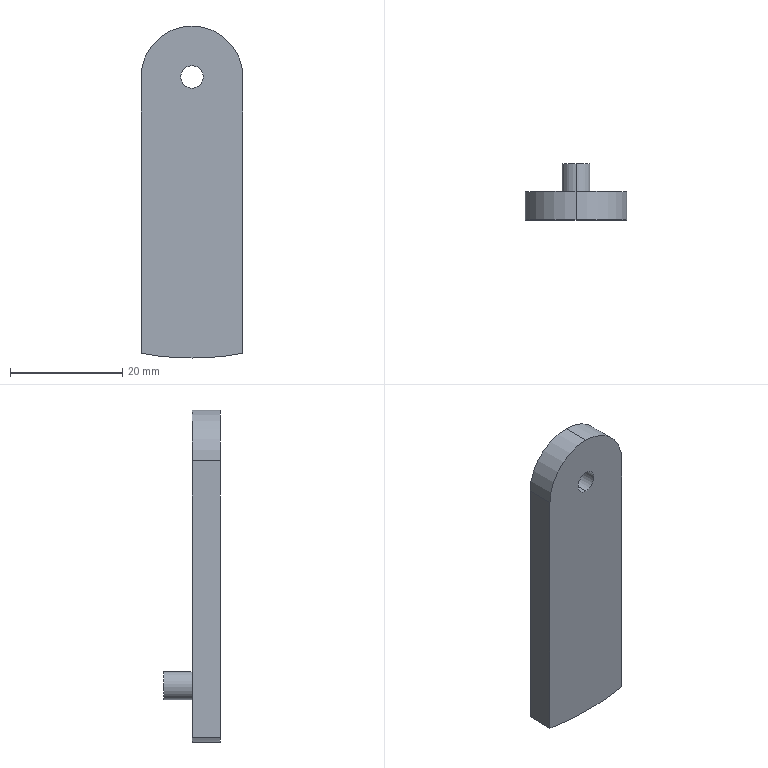Part | SolidWorks | features ICE 3, Extrusion 1 | 1 solid | 13 faces | box 18.129 x 10 x 59.065 mm | volume 5188 mm3 | cylinder 8 | plane 5 | commonest cylinder face diameters 4 x2 5 x2 18.129 x2 100 x2
STEP:
#1=CARTESIAN_POINT('',(0.,5.,-2.));
#2=VERTEX_POINT('',#1);
#3=CARTESIAN_POINT('',(0.,5.,2.));
#4=VERTEX_POINT('',#3);
#5=CARTESIAN_POINT('',(0.,5.,0.));
#6=DIRECTION('',(0.,1.,0.));
#7=DIRECTION('',(0.,0.,1.));
#8=AXIS2_PLACEMENT_3D('',#5,#6,#7);
#9=CIRCLE('',#8,2.);
#10=EDGE_CURVE('',#2,#4,#9,.T.);
#11=ORIENTED_EDGE('',*,*,#10,.T.);
#12=CARTESIAN_POINT('',(0.,0.,2.));
#13=VERTEX_POINT('',#12);
#14=CARTESIAN_POINT('',(0.,10.,2.));
#15=DIRECTION('',(0.,-1.,0.));
#16=VECTOR('',#15,1000.);
#17=LINE('',#14,#16);
#18=EDGE_CURVE('',#4,#13,#17,.T.);
#19=ORIENTED_EDGE('',*,*,#18,.T.);
#20=CARTESIAN_POINT('',(0.,0.,-2.));
#21=VERTEX_POINT('',#20);
#22=CARTESIAN_POINT('',(0.,0.,0.));
#23=DIRECTION('',(0.,-1.,0.));
#24=DIRECTION('',(0.,0.,-1.));
#25=AXIS2_PLACEMENT_3D('',#22,#23,#24);
#26=CIRCLE('',#25,2.);
#27=EDGE_CURVE('',#13,#21,#26,.T.);
#28=ORIENTED_EDGE('',*,*,#27,.T.);
#29=CARTESIAN_POINT('',(0.,10.,-2.));
#30=DIRECTION('',(0.,-1.,0.));
#31=VECTOR('',#30,1000.);
#32=LINE('',#29,#31);
#33=EDGE_CURVE('',#2,#21,#32,.T.);
#34=ORIENTED_EDGE('',*,*,#33,.F.);
#35=EDGE_LOOP('',(#11,#19,#28,#34));
#36=FACE_OUTER_BOUND('',#35,.T.);
#37=CARTESIAN_POINT('',(0.,10.,0.));
#38=DIRECTION('',(0.,-1.,0.));
#39=DIRECTION('',(0.,0.,-1.));
#40=AXIS2_PLACEMENT_3D('',#37,#38,#39);
#41=CYLINDRICAL_SURFACE('',#40,2.);
#42=ADVANCED_FACE('',(#36),#41,.F.);
#43=CARTESIAN_POINT('',(0.,0.,9.065));
#44=VERTEX_POINT('',#43);
#45=CARTESIAN_POINT('',(-9.065,0.,0.));
#46=VERTEX_POINT('',#45);
#47=CARTESIAN_POINT('',(0.,0.,0.));
#48=DIRECTION('',(0.,-1.,0.));
#49=DIRECTION('',(0.,0.,1.));
#50=AXIS2_PLACEMENT_3D('',#47,#48,#49);
#51=CIRCLE('',#50,9.065);
#52=EDGE_CURVE('',#44,#46,#51,.T.);
#53=ORIENTED_EDGE('',*,*,#52,.F.);
#54=CARTESIAN_POINT('',(0.,5.,9.065));
#55=VERTEX_POINT('',#54);
#56=CARTESIAN_POINT('',(0.,-6.,9.065));
#57=DIRECTION('',(0.,1.,0.));
#58=VECTOR('',#57,1000.);
#59=LINE('',#56,#58);
#60=EDGE_CURVE('',#44,#55,#59,.T.);
#61=ORIENTED_EDGE('',*,*,#60,.T.);
#62=CARTESIAN_POINT('',(-9.065,5.,0.));
#63=VERTEX_POINT('',#62);
#64=CARTESIAN_POINT('',(0.,5.,0.));
#65=DIRECTION('',(0.,-1.,0.));
#66=DIRECTION('',(0.,0.,1.));
#67=AXIS2_PLACEMENT_3D('',#64,#65,#66);
#68=CIRCLE('',#67,9.065);
#69=EDGE_CURVE('',#55,#63,#68,.T.);
#70=ORIENTED_EDGE('',*,*,#69,.T.);
#71=CARTESIAN_POINT('',(-9.065,-6.,0.));
#72=DIRECTION('',(0.,1.,0.));
#73=VECTOR('',#72,1000.);
#74=LINE('',#71,#73);
#75=EDGE_CURVE('',#46,#63,#74,.T.);
#76=ORIENTED_EDGE('',*,*,#75,.F.);
#77=EDGE_LOOP('',(#53,#61,#70,#76));
#78=FACE_OUTER_BOUND('',#77,.T.);
#79=CARTESIAN_POINT('',(0.,-6.,0.));
#80=DIRECTION('',(0.,1.,0.));
#81=DIRECTION('',(0.,0.,1.));
#82=AXIS2_PLACEMENT_3D('',#79,#80,#81);
#83=CYLINDRICAL_SURFACE('',#82,9.065);
#84=ADVANCED_FACE('',(#78),#83,.T.);
#85=CARTESIAN_POINT('',(0.,10.,-37.5));
#86=VERTEX_POINT('',#85);
#87=CARTESIAN_POINT('',(0.,10.,-42.5));
#88=VERTEX_POINT('',#87);
#89=CARTESIAN_POINT('',(0.,10.,-40.));
#90=DIRECTION('',(0.,1.,0.));
#91=DIRECTION('',(0.,0.,1.));
#92=AXIS2_PLACEMENT_3D('',#89,#90,#91);
#93=CIRCLE('',#92,2.5);
#94=EDGE_CURVE('',#86,#88,#93,.T.);
#95=ORIENTED_EDGE('',*,*,#94,.F.);
#96=CARTESIAN_POINT('',(0.,5.,-37.5));
#97=VERTEX_POINT('',#96);
#98=CARTESIAN_POINT('',(0.,10.,-37.5));
#99=DIRECTION('',(0.,-1.,0.));
#100=VECTOR('',#99,1000.);
#101=LINE('',#98,#100);
#102=EDGE_CURVE('',#86,#97,#101,.T.);
#103=ORIENTED_EDGE('',*,*,#102,.T.);
#104=CARTESIAN_POINT('',(0.,5.,-42.5));
#105=VERTEX_POINT('',#104);
#106=CARTESIAN_POINT('',(0.,5.,-40.));
#107=DIRECTION('',(0.,-1.,0.));
#108=DIRECTION('',(0.,0.,1.));
#109=AXIS2_PLACEMENT_3D('',#106,#107,#108);
#110=CIRCLE('',#109,2.5);
#111=EDGE_CURVE('',#105,#97,#110,.T.);
#112=ORIENTED_EDGE('',*,*,#111,.F.);
#113=CARTESIAN_POINT('',(0.,10.,-42.5));
#114=DIRECTION('',(0.,-1.,0.));
#115=VECTOR('',#114,1000.);
#116=LINE('',#113,#115);
#117=EDGE_CURVE('',#88,#105,#116,.T.);
#118=ORIENTED_EDGE('',*,*,#117,.F.);
#119=EDGE_LOOP('',(#95,#103,#112,#118));
#120=FACE_OUTER_BOUND('',#119,.T.);
#121=CARTESIAN_POINT('',(0.,10.,-40.));
#122=DIRECTION('',(0.,-1.,0.));
#123=DIRECTION('',(0.,0.,-1.));
#124=AXIS2_PLACEMENT_3D('',#121,#122,#123);
#125=CYLINDRICAL_SURFACE('',#124,2.5);
#126=ADVANCED_FACE('',(#120),#125,.T.);
#127=CARTESIAN_POINT('',(0.,5.,-50.));
#128=VERTEX_POINT('',#127);
#129=CARTESIAN_POINT('',(-9.065,5.,-49.171));
#130=VERTEX_POINT('',#129);
#131=CARTESIAN_POINT('',(0.,5.,0.));
#132=DIRECTION('',(0.,1.,0.));
#133=DIRECTION('',(0.,0.,1.));
#134=AXIS2_PLACEMENT_3D('',#131,#132,#133);
#135=CIRCLE('',#134,50.);
#136=EDGE_CURVE('',#128,#130,#135,.T.);
#137=ORIENTED_EDGE('',*,*,#136,.F.);
#138=CARTESIAN_POINT('',(0.,0.,-50.));
#139=VERTEX_POINT('',#138);
#140=CARTESIAN_POINT('',(0.,5.,-50.));
#141=DIRECTION('',(0.,-1.,0.));
#142=VECTOR('',#141,1000.);
#143=LINE('',#140,#142);
#144=EDGE_CURVE('',#128,#139,#143,.T.);
#145=ORIENTED_EDGE('',*,*,#144,.T.);
#146=CARTESIAN_POINT('',(-9.065,0.,-49.171));
#147=VERTEX_POINT('',#146);
#148=CARTESIAN_POINT('',(0.,0.,0.));
#149=DIRECTION('',(0.,1.,0.));
#150=DIRECTION('',(0.,0.,1.));
#151=AXIS2_PLACEMENT_3D('',#148,#149,#150);
#152=CIRCLE('',#151,50.);
#153=EDGE_CURVE('',#139,#147,#152,.T.);
#154=ORIENTED_EDGE('',*,*,#153,.T.);
#155=CARTESIAN_POINT('',(-9.065,-6.,-49.171));
#156=DIRECTION('',(0.,1.,0.));
#157=VECTOR('',#156,1000.);
#158=LINE('',#155,#157);
#159=EDGE_CURVE('',#147,#130,#158,.T.);
#160=ORIENTED_EDGE('',*,*,#159,.T.);
#161=EDGE_LOOP('',(#137,#145,#154,#160));
#162=FACE_OUTER_BOUND('',#161,.T.);
#163=CARTESIAN_POINT('',(0.,5.,0.));
#164=DIRECTION('',(0.,-1.,0.));
#165=DIRECTION('',(0.,0.,-1.));
#166=AXIS2_PLACEMENT_3D('',#163,#164,#165);
#167=CYLINDRICAL_SURFACE('',#166,50.);
#168=ADVANCED_FACE('',(#162),#167,.T.);
#169=ORIENTED_EDGE('',*,*,#144,.F.);
#170=CARTESIAN_POINT('',(9.065,5.,-49.171));
#171=VERTEX_POINT('',#170);
#172=CARTESIAN_POINT('',(0.,5.,0.));
#173=DIRECTION('',(0.,1.,0.));
#174=DIRECTION('',(0.,0.,1.));
#175=AXIS2_PLACEMENT_3D('',#172,#173,#174);
#176=CIRCLE('',#175,50.);
#177=EDGE_CURVE('',#171,#128,#176,.T.);
#178=ORIENTED_EDGE('',*,*,#177,.F.);
#179=CARTESIAN_POINT('',(9.065,0.,-49.171));
#180=VERTEX_POINT('',#179);
#181=CARTESIAN_POINT('',(9.065,-6.,-49.171));
#182=DIRECTION('',(0.,1.,0.));
#183=VECTOR('',#182,1000.);
#184=LINE('',#181,#183);
#185=EDGE_CURVE('',#180,#171,#184,.T.);
#186=ORIENTED_EDGE('',*,*,#185,.F.);
#187=CARTESIAN_POINT('',(0.,0.,0.));
#188=DIRECTION('',(0.,1.,0.));
#189=DIRECTION('',(0.,0.,1.));
#190=AXIS2_PLACEMENT_3D('',#187,#188,#189);
#191=CIRCLE('',#190,50.);
#192=EDGE_CURVE('',#180,#139,#191,.T.);
#193=ORIENTED_EDGE('',*,*,#192,.T.);
#194=EDGE_LOOP('',(#169,#178,#186,#193));
#195=FACE_OUTER_BOUND('',#194,.T.);
#196=CARTESIAN_POINT('',(0.,5.,0.));
#197=DIRECTION('',(0.,-1.,0.));
#198=DIRECTION('',(0.,0.,-1.));
#199=AXIS2_PLACEMENT_3D('',#196,#197,#198);
#200=CYLINDRICAL_SURFACE('',#199,50.);
#201=ADVANCED_FACE('',(#195),#200,.T.);
#202=ORIENTED_EDGE('',*,*,#10,.F.);
#203=CARTESIAN_POINT('',(0.,5.,0.));
#204=DIRECTION('',(0.,1.,0.));
#205=DIRECTION('',(0.,0.,1.));
#206=AXIS2_PLACEMENT_3D('',#203,#204,#205);
#207=CIRCLE('',#206,2.);
#208=EDGE_CURVE('',#4,#2,#207,.T.);
#209=ORIENTED_EDGE('',*,*,#208,.F.);
#210=EDGE_LOOP('',(#202,#209));
#211=FACE_BOUND('',#210,.T.);
#212=CARTESIAN_POINT('',(-9.065,5.,-20.));
#213=DIRECTION('',(0.,0.,-1.));
#214=VECTOR('',#213,1000.);
#215=LINE('',#212,#214);
#216=EDGE_CURVE('',#63,#130,#215,.T.);
#217=ORIENTED_EDGE('',*,*,#216,.F.);
#218=ORIENTED_EDGE('',*,*,#69,.F.);
#219=CARTESIAN_POINT('',(9.065,5.,0.));
#220=VERTEX_POINT('',#219);
#221=CARTESIAN_POINT('',(0.,5.,0.));
#222=DIRECTION('',(0.,-1.,0.));
#223=DIRECTION('',(0.,0.,1.));
#224=AXIS2_PLACEMENT_3D('',#221,#222,#223);
#225=CIRCLE('',#224,9.065);
#226=EDGE_CURVE('',#220,#55,#225,.T.);
#227=ORIENTED_EDGE('',*,*,#226,.F.);
#228=CARTESIAN_POINT('',(9.065,5.,-20.));
#229=DIRECTION('',(0.,0.,1.));
#230=VECTOR('',#229,1000.);
#231=LINE('',#228,#230);
#232=EDGE_CURVE('',#171,#220,#231,.T.);
#233=ORIENTED_EDGE('',*,*,#232,.F.);
#234=ORIENTED_EDGE('',*,*,#177,.T.);
#235=ORIENTED_EDGE('',*,*,#136,.T.);
#236=EDGE_LOOP('',(#217,#218,#227,#233,#234,#235));
#237=FACE_OUTER_BOUND('',#236,.T.);
#238=ORIENTED_EDGE('',*,*,#111,.T.);
#239=CARTESIAN_POINT('',(0.,5.,-40.));
#240=DIRECTION('',(0.,-1.,0.));
#241=DIRECTION('',(0.,0.,1.));
#242=AXIS2_PLACEMENT_3D('',#239,#240,#241);
#243=CIRCLE('',#242,2.5);
#244=EDGE_CURVE('',#97,#105,#243,.T.);
#245=ORIENTED_EDGE('',*,*,#244,.T.);
#246=EDGE_LOOP('',(#238,#245));
#247=FACE_BOUND('',#246,.T.);
#248=CARTESIAN_POINT('',(0.,5.,0.));
#249=DIRECTION('',(0.,1.,0.));
#250=DIRECTION('',(0.,0.,1.));
#251=AXIS2_PLACEMENT_3D('',#248,#249,#250);
#252=PLANE('',#251);
#253=ADVANCED_FACE('',(#211,#237,#247),#252,.T.);
#254=CARTESIAN_POINT('',(0.,0.,0.));
#255=DIRECTION('',(0.,-1.,0.));
#256=DIRECTION('',(0.,0.,-1.));
#257=AXIS2_PLACEMENT_3D('',#254,#255,#256);
#258=CIRCLE('',#257,2.);
#259=EDGE_CURVE('',#21,#13,#258,.T.);
#260=ORIENTED_EDGE('',*,*,#259,.F.);
#261=ORIENTED_EDGE('',*,*,#27,.F.);
#262=EDGE_LOOP('',(#260,#261));
#263=FACE_BOUND('',#262,.T.);
#264=CARTESIAN_POINT('',(9.065,0.,0.));
#265=VERTEX_POINT('',#264);
#266=CARTESIAN_POINT('',(0.,0.,0.));
#267=DIRECTION('',(0.,-1.,0.));
#268=DIRECTION('',(0.,0.,1.));
#269=AXIS2_PLACEMENT_3D('',#266,#267,#268);
#270=CIRCLE('',#269,9.065);
#271=EDGE_CURVE('',#265,#44,#270,.T.);
#272=ORIENTED_EDGE('',*,*,#271,.T.);
#273=ORIENTED_EDGE('',*,*,#52,.T.);
#274=CARTESIAN_POINT('',(-9.065,0.,0.));
#275=DIRECTION('',(0.,0.,-1.));
#276=VECTOR('',#275,1000.);
#277=LINE('',#274,#276);
#278=EDGE_CURVE('',#46,#147,#277,.T.);
#279=ORIENTED_EDGE('',*,*,#278,.T.);
#280=ORIENTED_EDGE('',*,*,#153,.F.);
#281=ORIENTED_EDGE('',*,*,#192,.F.);
#282=CARTESIAN_POINT('',(9.065,0.,0.));
#283=DIRECTION('',(0.,0.,1.));
#284=VECTOR('',#283,1000.);
#285=LINE('',#282,#284);
#286=EDGE_CURVE('',#180,#265,#285,.T.);
#287=ORIENTED_EDGE('',*,*,#286,.T.);
#288=EDGE_LOOP('',(#272,#273,#279,#280,#281,#287));
#289=FACE_OUTER_BOUND('',#288,.T.);
#290=CARTESIAN_POINT('',(0.,0.,0.));
#291=DIRECTION('',(0.,1.,0.));
#292=DIRECTION('',(0.,0.,1.));
#293=AXIS2_PLACEMENT_3D('',#290,#291,#292);
#294=PLANE('',#293);
#295=ADVANCED_FACE('',(#263,#289),#294,.F.);
#296=ORIENTED_EDGE('',*,*,#102,.F.);
#297=CARTESIAN_POINT('',(0.,10.,-40.));
#298=DIRECTION('',(0.,1.,0.));
#299=DIRECTION('',(0.,0.,1.));
#300=AXIS2_PLACEMENT_3D('',#297,#298,#299);
#301=CIRCLE('',#300,2.5);
#302=EDGE_CURVE('',#88,#86,#301,.T.);
#303=ORIENTED_EDGE('',*,*,#302,.F.);
#304=ORIENTED_EDGE('',*,*,#117,.T.);
#305=ORIENTED_EDGE('',*,*,#244,.F.);
#306=EDGE_LOOP('',(#296,#303,#304,#305));
#307=FACE_OUTER_BOUND('',#306,.T.);
#308=CARTESIAN_POINT('',(0.,10.,-40.));
#309=DIRECTION('',(0.,-1.,0.));
#310=DIRECTION('',(0.,0.,-1.));
#311=AXIS2_PLACEMENT_3D('',#308,#309,#310);
#312=CYLINDRICAL_SURFACE('',#311,2.5);
#313=ADVANCED_FACE('',(#307),#312,.T.);
#314=ORIENTED_EDGE('',*,*,#302,.T.);
#315=ORIENTED_EDGE('',*,*,#94,.T.);
#316=EDGE_LOOP('',(#314,#315));
#317=FACE_OUTER_BOUND('',#316,.T.);
#318=CARTESIAN_POINT('',(0.,10.,0.));
#319=DIRECTION('',(0.,1.,0.));
#320=DIRECTION('',(0.,0.,1.));
#321=AXIS2_PLACEMENT_3D('',#318,#319,#320);
#322=PLANE('',#321);
#323=ADVANCED_FACE('',(#317),#322,.T.);
#324=ORIENTED_EDGE('',*,*,#75,.T.);
#325=ORIENTED_EDGE('',*,*,#216,.T.);
#326=ORIENTED_EDGE('',*,*,#159,.F.);
#327=ORIENTED_EDGE('',*,*,#278,.F.);
#328=EDGE_LOOP('',(#324,#325,#326,#327));
#329=FACE_OUTER_BOUND('',#328,.T.);
#330=CARTESIAN_POINT('',(-9.065,-6.,-20.));
#331=DIRECTION('',(1.,0.,0.));
#332=DIRECTION('',(0.,0.,-1.));
#333=AXIS2_PLACEMENT_3D('',#330,#331,#332);
#334=PLANE('',#333);
#335=ADVANCED_FACE('',(#329),#334,.F.);
#336=ORIENTED_EDGE('',*,*,#60,.F.);
#337=ORIENTED_EDGE('',*,*,#271,.F.);
#338=CARTESIAN_POINT('',(9.065,-6.,0.));
#339=DIRECTION('',(0.,1.,0.));
#340=VECTOR('',#339,1000.);
#341=LINE('',#338,#340);
#342=EDGE_CURVE('',#265,#220,#341,.T.);
#343=ORIENTED_EDGE('',*,*,#342,.T.);
#344=ORIENTED_EDGE('',*,*,#226,.T.);
#345=EDGE_LOOP('',(#336,#337,#343,#344));
#346=FACE_OUTER_BOUND('',#345,.T.);
#347=CARTESIAN_POINT('',(0.,-6.,0.));
#348=DIRECTION('',(0.,1.,0.));
#349=DIRECTION('',(0.,0.,1.));
#350=AXIS2_PLACEMENT_3D('',#347,#348,#349);
#351=CYLINDRICAL_SURFACE('',#350,9.065);
#352=ADVANCED_FACE('',(#346),#351,.T.);
#353=ORIENTED_EDGE('',*,*,#185,.T.);
#354=ORIENTED_EDGE('',*,*,#232,.T.);
#355=ORIENTED_EDGE('',*,*,#342,.F.);
#356=ORIENTED_EDGE('',*,*,#286,.F.);
#357=EDGE_LOOP('',(#353,#354,#355,#356));
#358=FACE_OUTER_BOUND('',#357,.T.);
#359=CARTESIAN_POINT('',(9.065,-6.,-20.));
#360=DIRECTION('',(-1.,0.,0.));
#361=DIRECTION('',(0.,0.,1.));
#362=AXIS2_PLACEMENT_3D('',#359,#360,#361);
#363=PLANE('',#362);
#364=ADVANCED_FACE('',(#358),#363,.F.);
#365=ORIENTED_EDGE('',*,*,#18,.F.);
#366=ORIENTED_EDGE('',*,*,#208,.T.);
#367=ORIENTED_EDGE('',*,*,#33,.T.);
#368=ORIENTED_EDGE('',*,*,#259,.T.);
#369=EDGE_LOOP('',(#365,#366,#367,#368));
#370=FACE_OUTER_BOUND('',#369,.T.);
#371=CARTESIAN_POINT('',(0.,10.,0.));
#372=DIRECTION('',(0.,-1.,0.));
#373=DIRECTION('',(0.,0.,-1.));
#374=AXIS2_PLACEMENT_3D('',#371,#372,#373);
#375=CYLINDRICAL_SURFACE('',#374,2.);
#376=ADVANCED_FACE('',(#370),#375,.F.);
#377=CLOSED_SHELL('',(#42,#84,#126,#168,#201,#253,#295,#313,#323,#335,#352,#364,#376));
#378=MANIFOLD_SOLID_BREP('',#377);
#379=CARTESIAN_POINT('',(0.,0.,0.));
#380=DIRECTION('',(0.,0.,1.));
#381=DIRECTION('',(1.,0.,0.));
#382=AXIS2_PLACEMENT_3D('',#379,#380,#381);
#383=(LENGTH_UNIT()NAMED_UNIT(*)SI_UNIT(.MILLI.,.METRE.));
#384=UNCERTAINTY_MEASURE_WITH_UNIT(LENGTH_MEASURE(0.00001),#383,'','');
#385=(NAMED_UNIT(*)PLANE_ANGLE_UNIT()SI_UNIT($,.RADIAN.));
#386=(NAMED_UNIT(*)SI_UNIT($,.STERADIAN.)SOLID_ANGLE_UNIT());
#387=(GEOMETRIC_REPRESENTATION_CONTEXT(3)GLOBAL_UNCERTAINTY_ASSIGNED_CONTEXT((#384))GLOBAL_UNIT_ASSIGNED_CONTEXT((#383,#385,#386))REPRESENTATION_CONTEXT('',''));
#388=ADVANCED_BREP_SHAPE_REPRESENTATION('',(#378,#382),#387);